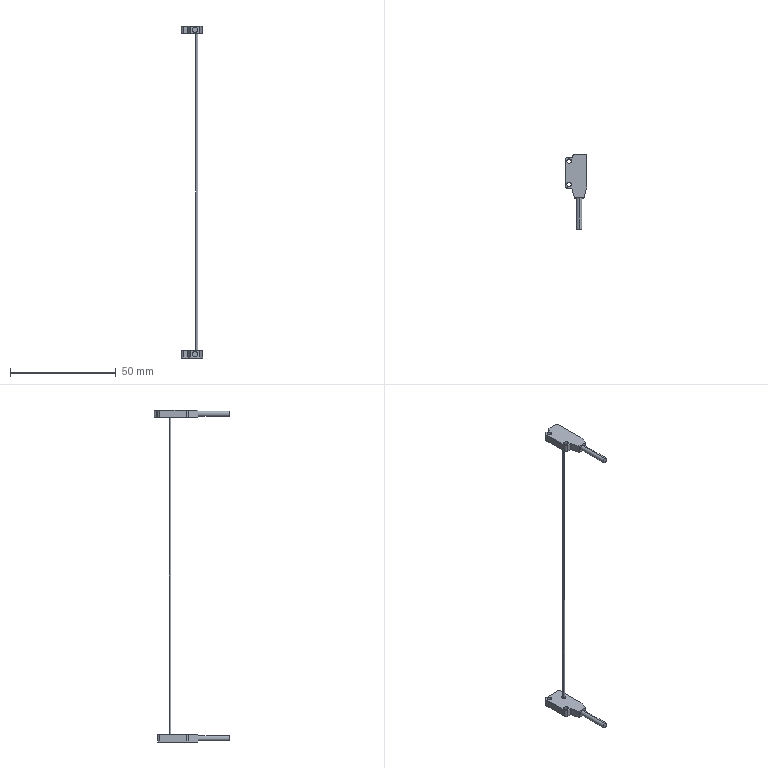Part | STEP file | Through-beam ultra-thin photoelectric switch EX-11A_150 | 2 solids | 50 faces | box 10 x 35.5 x 157 mm | volume 1436 mm3 | cylinder 25 | plane 25 | commonest cylinder face diameters 2 x11 2.2 x8 2.5 x4 1 x2